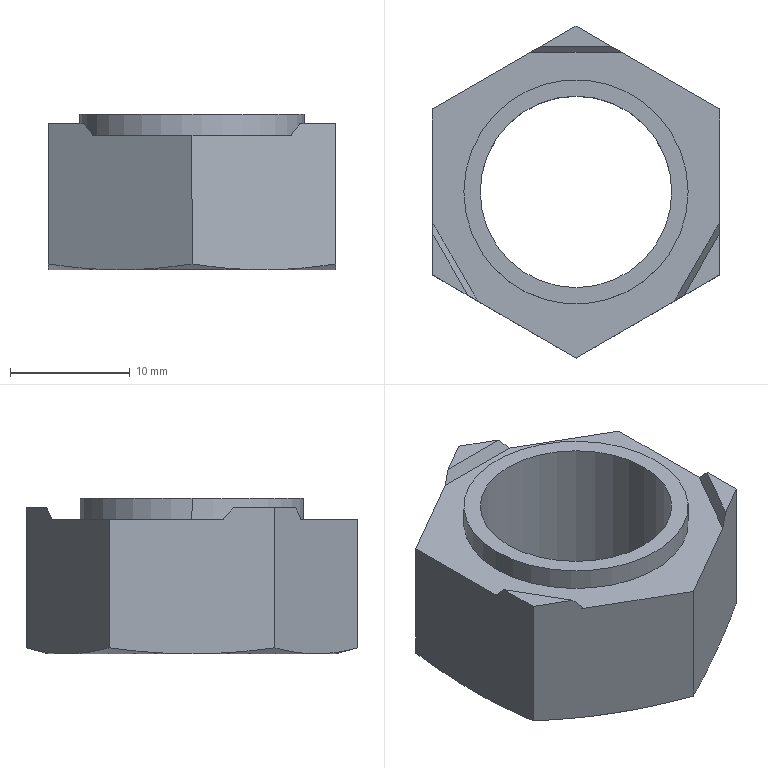Part | SolidWorks | features Cut 3, Boss 1, CirPattern 1, Extrusion 1, RefAxis 1 | 1 solid | 28 faces | box 24 x 27.713 x 13 mm | volume 3465 mm3 | plane 16 | cylinder 6 | cone 6 | commonest cylinder face diameters 16 x2 18.735 x2 19.13 x2
STEP:
#1=CARTESIAN_POINT('',(9.565,0.,0.2));
#2=VERTEX_POINT('',#1);
#3=CARTESIAN_POINT('',(-9.565,0.,0.2));
#4=VERTEX_POINT('',#3);
#5=CARTESIAN_POINT('',(0.,0.,0.2));
#6=DIRECTION('',(0.,0.,-1.));
#7=DIRECTION('',(-1.,0.,0.));
#8=AXIS2_PLACEMENT_3D('',#5,#6,#7);
#9=CIRCLE('',#8,9.565);
#10=EDGE_CURVE('',#2,#4,#9,.T.);
#11=ORIENTED_EDGE('',*,*,#10,.F.);
#12=CARTESIAN_POINT('',(9.565,0.,0.));
#13=VERTEX_POINT('',#12);
#14=CARTESIAN_POINT('',(9.565,0.,0.2));
#15=DIRECTION('',(0.,0.,-1.));
#16=VECTOR('',#15,1000.);
#17=LINE('',#14,#16);
#18=EDGE_CURVE('',#2,#13,#17,.T.);
#19=ORIENTED_EDGE('',*,*,#18,.T.);
#20=CARTESIAN_POINT('',(-9.565,0.,0.));
#21=VERTEX_POINT('',#20);
#22=CARTESIAN_POINT('',(0.,0.,0.));
#23=DIRECTION('',(0.,0.,-1.));
#24=DIRECTION('',(-1.,0.,0.));
#25=AXIS2_PLACEMENT_3D('',#22,#23,#24);
#26=CIRCLE('',#25,9.565);
#27=EDGE_CURVE('',#13,#21,#26,.T.);
#28=ORIENTED_EDGE('',*,*,#27,.T.);
#29=CARTESIAN_POINT('',(-9.565,0.,0.2));
#30=DIRECTION('',(0.,0.,-1.));
#31=VECTOR('',#30,1000.);
#32=LINE('',#29,#31);
#33=EDGE_CURVE('',#4,#21,#32,.T.);
#34=ORIENTED_EDGE('',*,*,#33,.F.);
#35=EDGE_LOOP('',(#11,#19,#28,#34));
#36=FACE_OUTER_BOUND('',#35,.T.);
#37=CARTESIAN_POINT('',(0.,0.,0.2));
#38=DIRECTION('',(0.,0.,-1.));
#39=DIRECTION('',(-1.,0.,0.));
#40=AXIS2_PLACEMENT_3D('',#37,#38,#39);
#41=CYLINDRICAL_SURFACE('',#40,9.565);
#42=ADVANCED_FACE('',(#36),#41,.F.);
#43=CARTESIAN_POINT('',(9.368,0.,13.));
#44=VERTEX_POINT('',#43);
#45=CARTESIAN_POINT('',(-9.367,0.,13.));
#46=VERTEX_POINT('',#45);
#47=CARTESIAN_POINT('',(0.,0.,13.));
#48=DIRECTION('',(0.,0.,1.));
#49=DIRECTION('',(1.,0.,0.));
#50=AXIS2_PLACEMENT_3D('',#47,#48,#49);
#51=CIRCLE('',#50,9.367);
#52=EDGE_CURVE('',#44,#46,#51,.T.);
#53=ORIENTED_EDGE('',*,*,#52,.F.);
#54=CARTESIAN_POINT('',(9.368,0.,11.2));
#55=VERTEX_POINT('',#54);
#56=CARTESIAN_POINT('',(9.367,0.,13.));
#57=DIRECTION('',(0.,0.,-1.));
#58=VECTOR('',#57,1000.);
#59=LINE('',#56,#58);
#60=EDGE_CURVE('',#44,#55,#59,.T.);
#61=ORIENTED_EDGE('',*,*,#60,.T.);
#62=CARTESIAN_POINT('',(-9.367,0.,11.2));
#63=VERTEX_POINT('',#62);
#64=CARTESIAN_POINT('',(0.,0.,11.2));
#65=DIRECTION('',(0.,0.,1.));
#66=DIRECTION('',(-1.,0.,0.));
#67=AXIS2_PLACEMENT_3D('',#64,#65,#66);
#68=CIRCLE('',#67,9.367);
#69=EDGE_CURVE('',#55,#63,#68,.T.);
#70=ORIENTED_EDGE('',*,*,#69,.T.);
#71=CARTESIAN_POINT('',(-9.367,0.,13.));
#72=DIRECTION('',(0.,0.,-1.));
#73=VECTOR('',#72,1000.);
#74=LINE('',#71,#73);
#75=EDGE_CURVE('',#46,#63,#74,.T.);
#76=ORIENTED_EDGE('',*,*,#75,.F.);
#77=EDGE_LOOP('',(#53,#61,#70,#76));
#78=FACE_OUTER_BOUND('',#77,.T.);
#79=CARTESIAN_POINT('',(0.,0.,13.));
#80=DIRECTION('',(0.,0.,-1.));
#81=DIRECTION('',(-1.,0.,0.));
#82=AXIS2_PLACEMENT_3D('',#79,#80,#81);
#83=CYLINDRICAL_SURFACE('',#82,9.367);
#84=ADVANCED_FACE('',(#78),#83,.T.);
#85=CARTESIAN_POINT('',(-8.,0.,13.));
#86=VERTEX_POINT('',#85);
#87=CARTESIAN_POINT('',(8.,0.,13.));
#88=VERTEX_POINT('',#87);
#89=CARTESIAN_POINT('',(0.,0.,13.));
#90=DIRECTION('',(0.,0.,1.));
#91=DIRECTION('',(1.,0.,0.));
#92=AXIS2_PLACEMENT_3D('',#89,#90,#91);
#93=CIRCLE('',#92,8.);
#94=EDGE_CURVE('',#86,#88,#93,.T.);
#95=ORIENTED_EDGE('',*,*,#94,.T.);
#96=CARTESIAN_POINT('',(8.,0.,0.2));
#97=VERTEX_POINT('',#96);
#98=CARTESIAN_POINT('',(8.,0.,13.));
#99=DIRECTION('',(0.,0.,-1.));
#100=VECTOR('',#99,1000.);
#101=LINE('',#98,#100);
#102=EDGE_CURVE('',#88,#97,#101,.T.);
#103=ORIENTED_EDGE('',*,*,#102,.T.);
#104=CARTESIAN_POINT('',(-8.,0.,0.2));
#105=VERTEX_POINT('',#104);
#106=CARTESIAN_POINT('',(0.,0.,0.2));
#107=DIRECTION('',(0.,0.,-1.));
#108=DIRECTION('',(-1.,0.,0.));
#109=AXIS2_PLACEMENT_3D('',#106,#107,#108);
#110=CIRCLE('',#109,8.);
#111=EDGE_CURVE('',#97,#105,#110,.T.);
#112=ORIENTED_EDGE('',*,*,#111,.T.);
#113=CARTESIAN_POINT('',(-8.,0.,13.));
#114=DIRECTION('',(0.,0.,-1.));
#115=VECTOR('',#114,1000.);
#116=LINE('',#113,#115);
#117=EDGE_CURVE('',#86,#105,#116,.T.);
#118=ORIENTED_EDGE('',*,*,#117,.F.);
#119=EDGE_LOOP('',(#95,#103,#112,#118));
#120=FACE_OUTER_BOUND('',#119,.T.);
#121=CARTESIAN_POINT('',(0.,0.,13.));
#122=DIRECTION('',(0.,0.,-1.));
#123=DIRECTION('',(-1.,0.,0.));
#124=AXIS2_PLACEMENT_3D('',#121,#122,#123);
#125=CYLINDRICAL_SURFACE('',#124,8.);
#126=ADVANCED_FACE('',(#120),#125,.F.);
#127=ORIENTED_EDGE('',*,*,#102,.F.);
#128=CARTESIAN_POINT('',(0.,0.,13.));
#129=DIRECTION('',(0.,0.,1.));
#130=DIRECTION('',(1.,0.,0.));
#131=AXIS2_PLACEMENT_3D('',#128,#129,#130);
#132=CIRCLE('',#131,8.);
#133=EDGE_CURVE('',#88,#86,#132,.T.);
#134=ORIENTED_EDGE('',*,*,#133,.T.);
#135=ORIENTED_EDGE('',*,*,#117,.T.);
#136=CARTESIAN_POINT('',(0.,0.,0.2));
#137=DIRECTION('',(0.,0.,-1.));
#138=DIRECTION('',(-1.,0.,0.));
#139=AXIS2_PLACEMENT_3D('',#136,#137,#138);
#140=CIRCLE('',#139,8.);
#141=EDGE_CURVE('',#105,#97,#140,.T.);
#142=ORIENTED_EDGE('',*,*,#141,.T.);
#143=EDGE_LOOP('',(#127,#134,#135,#142));
#144=FACE_OUTER_BOUND('',#143,.T.);
#145=CARTESIAN_POINT('',(0.,0.,13.));
#146=DIRECTION('',(0.,0.,-1.));
#147=DIRECTION('',(-1.,0.,0.));
#148=AXIS2_PLACEMENT_3D('',#145,#146,#147);
#149=CYLINDRICAL_SURFACE('',#148,8.);
#150=ADVANCED_FACE('',(#144),#149,.F.);
#151=CARTESIAN_POINT('',(0.,0.,0.));
#152=DIRECTION('',(0.,0.,-1.));
#153=DIRECTION('',(-1.,0.,0.));
#154=AXIS2_PLACEMENT_3D('',#151,#152,#153);
#155=CIRCLE('',#154,9.565);
#156=EDGE_CURVE('',#21,#13,#155,.T.);
#157=ORIENTED_EDGE('',*,*,#156,.F.);
#158=ORIENTED_EDGE('',*,*,#27,.F.);
#159=EDGE_LOOP('',(#157,#158));
#160=FACE_BOUND('',#159,.T.);
#161=CARTESIAN_POINT('',(-6.,-10.392,0.));
#162=VERTEX_POINT('',#161);
#163=CARTESIAN_POINT('',(-12.,0.,0.));
#164=VERTEX_POINT('',#163);
#165=CARTESIAN_POINT('',(0.,0.,0.));
#166=DIRECTION('',(0.,0.,-1.));
#167=DIRECTION('',(-1.,0.,0.));
#168=AXIS2_PLACEMENT_3D('',#165,#166,#167);
#169=CIRCLE('',#168,12.);
#170=EDGE_CURVE('',#162,#164,#169,.T.);
#171=ORIENTED_EDGE('',*,*,#170,.T.);
#172=CARTESIAN_POINT('',(-6.,10.392,0.));
#173=VERTEX_POINT('',#172);
#174=CARTESIAN_POINT('',(0.,0.,0.));
#175=DIRECTION('',(0.,0.,-1.));
#176=DIRECTION('',(-1.,0.,0.));
#177=AXIS2_PLACEMENT_3D('',#174,#175,#176);
#178=CIRCLE('',#177,12.);
#179=EDGE_CURVE('',#164,#173,#178,.T.);
#180=ORIENTED_EDGE('',*,*,#179,.T.);
#181=CARTESIAN_POINT('',(6.,10.392,0.));
#182=VERTEX_POINT('',#181);
#183=CARTESIAN_POINT('',(0.,0.,0.));
#184=DIRECTION('',(0.,0.,-1.));
#185=DIRECTION('',(-1.,0.,0.));
#186=AXIS2_PLACEMENT_3D('',#183,#184,#185);
#187=CIRCLE('',#186,12.);
#188=EDGE_CURVE('',#173,#182,#187,.T.);
#189=ORIENTED_EDGE('',*,*,#188,.T.);
#190=CARTESIAN_POINT('',(12.,0.,0.));
#191=VERTEX_POINT('',#190);
#192=CARTESIAN_POINT('',(0.,0.,0.));
#193=DIRECTION('',(0.,0.,-1.));
#194=DIRECTION('',(-1.,0.,0.));
#195=AXIS2_PLACEMENT_3D('',#192,#193,#194);
#196=CIRCLE('',#195,12.);
#197=EDGE_CURVE('',#182,#191,#196,.T.);
#198=ORIENTED_EDGE('',*,*,#197,.T.);
#199=CARTESIAN_POINT('',(6.,-10.392,0.));
#200=VERTEX_POINT('',#199);
#201=CARTESIAN_POINT('',(0.,0.,0.));
#202=DIRECTION('',(0.,0.,-1.));
#203=DIRECTION('',(-1.,0.,0.));
#204=AXIS2_PLACEMENT_3D('',#201,#202,#203);
#205=CIRCLE('',#204,12.);
#206=EDGE_CURVE('',#191,#200,#205,.T.);
#207=ORIENTED_EDGE('',*,*,#206,.T.);
#208=CARTESIAN_POINT('',(0.,0.,0.));
#209=DIRECTION('',(0.,0.,-1.));
#210=DIRECTION('',(-1.,0.,0.));
#211=AXIS2_PLACEMENT_3D('',#208,#209,#210);
#212=CIRCLE('',#211,12.);
#213=EDGE_CURVE('',#200,#162,#212,.T.);
#214=ORIENTED_EDGE('',*,*,#213,.T.);
#215=EDGE_LOOP('',(#171,#180,#189,#198,#207,#214));
#216=FACE_OUTER_BOUND('',#215,.T.);
#217=CARTESIAN_POINT('',(12.,6.928,0.));
#218=DIRECTION('',(0.,0.,-1.));
#219=DIRECTION('',(-1.,0.,0.));
#220=AXIS2_PLACEMENT_3D('',#217,#218,#219);
#221=PLANE('',#220);
#222=ADVANCED_FACE('',(#160,#216),#221,.T.);
#223=CARTESIAN_POINT('',(0.,13.856,0.4974));
#224=VERTEX_POINT('',#223);
#225=CARTESIAN_POINT('',(0.,13.856,0.4974));
#226=CARTESIAN_POINT('',(1.,13.279,0.3427));
#227=CARTESIAN_POINT('',(2.,12.702,0.2171));
#228=CARTESIAN_POINT('',(4.,11.547,0.04548));
#229=CARTESIAN_POINT('',(5.,10.97,0.));
#230=CARTESIAN_POINT('',(6.,10.392,0.));
#231=B_SPLINE_CURVE_WITH_KNOTS('',3,(#225,#226,#227,#228,#229,#230),.UNSPECIFIED.,.F.,.F.,(4,2,4),(0.000000231,0.003464,0.006928),.UNSPECIFIED.);
#232=EDGE_CURVE('',#224,#182,#231,.T.);
#233=ORIENTED_EDGE('',*,*,#232,.F.);
#234=CARTESIAN_POINT('',(0.,13.856,12.2));
#235=VERTEX_POINT('',#234);
#236=CARTESIAN_POINT('',(0.,13.856,13.));
#237=DIRECTION('',(0.,0.,-1.));
#238=VECTOR('',#237,1000.);
#239=LINE('',#236,#238);
#240=EDGE_CURVE('',#235,#224,#239,.T.);
#241=ORIENTED_EDGE('',*,*,#240,.F.);
#242=CARTESIAN_POINT('',(2.985,12.133,12.2));
#243=VERTEX_POINT('',#242);
#244=CARTESIAN_POINT('',(12.,6.928,12.2));
#245=DIRECTION('',(0.866,-0.5,0.));
#246=VECTOR('',#245,1000.);
#247=LINE('',#244,#246);
#248=EDGE_CURVE('',#235,#243,#247,.T.);
#249=ORIENTED_EDGE('',*,*,#248,.T.);
#250=CARTESIAN_POINT('',(3.793,11.667,11.2));
#251=VERTEX_POINT('',#250);
#252=CARTESIAN_POINT('',(6.833,9.911,7.436));
#253=DIRECTION('',(0.5907,-0.341,-0.7313));
#254=VECTOR('',#253,1000.);
#255=LINE('',#252,#254);
#256=EDGE_CURVE('',#243,#251,#255,.T.);
#257=ORIENTED_EDGE('',*,*,#256,.T.);
#258=CARTESIAN_POINT('',(12.,6.928,11.2));
#259=VERTEX_POINT('',#258);
#260=CARTESIAN_POINT('',(12.,6.928,11.2));
#261=DIRECTION('',(0.866,-0.5,0.));
#262=VECTOR('',#261,1000.);
#263=LINE('',#260,#262);
#264=EDGE_CURVE('',#251,#259,#263,.T.);
#265=ORIENTED_EDGE('',*,*,#264,.T.);
#266=CARTESIAN_POINT('',(12.,6.928,0.4974));
#267=VERTEX_POINT('',#266);
#268=CARTESIAN_POINT('',(12.,6.928,13.));
#269=DIRECTION('',(0.,0.,-1.));
#270=VECTOR('',#269,1000.);
#271=LINE('',#268,#270);
#272=EDGE_CURVE('',#259,#267,#271,.T.);
#273=ORIENTED_EDGE('',*,*,#272,.T.);
#274=CARTESIAN_POINT('',(6.,10.392,0.));
#275=CARTESIAN_POINT('',(7.,9.815,0.));
#276=CARTESIAN_POINT('',(8.,9.238,0.04548));
#277=CARTESIAN_POINT('',(10.,8.083,0.2171));
#278=CARTESIAN_POINT('',(11.,7.506,0.3427));
#279=CARTESIAN_POINT('',(12.,6.928,0.4974));
#280=B_SPLINE_CURVE_WITH_KNOTS('',3,(#274,#275,#276,#277,#278,#279),.UNSPECIFIED.,.F.,.F.,(4,2,4),(0.006928,0.01039,0.01386),.UNSPECIFIED.);
#281=EDGE_CURVE('',#182,#267,#280,.T.);
#282=ORIENTED_EDGE('',*,*,#281,.F.);
#283=EDGE_LOOP('',(#233,#241,#249,#257,#265,#273,#282));
#284=FACE_OUTER_BOUND('',#283,.T.);
#285=CARTESIAN_POINT('',(12.,6.928,13.));
#286=DIRECTION('',(-0.5,-0.866,0.));
#287=DIRECTION('',(0.866,-0.5,0.));
#288=AXIS2_PLACEMENT_3D('',#285,#286,#287);
#289=PLANE('',#288);
#290=ADVANCED_FACE('',(#284),#289,.F.);
#291=CARTESIAN_POINT('',(-12.,6.928,0.4974));
#292=VERTEX_POINT('',#291);
#293=CARTESIAN_POINT('',(-12.,6.928,0.4974));
#294=CARTESIAN_POINT('',(-11.,7.506,0.3427));
#295=CARTESIAN_POINT('',(-10.,8.083,0.2171));
#296=CARTESIAN_POINT('',(-8.,9.238,0.04548));
#297=CARTESIAN_POINT('',(-7.,9.815,0.));
#298=CARTESIAN_POINT('',(-6.,10.392,0.));
#299=B_SPLINE_CURVE_WITH_KNOTS('',3,(#293,#294,#295,#296,#297,#298),.UNSPECIFIED.,.F.,.F.,(4,2,4),(0.000000231,0.003464,0.006928),.UNSPECIFIED.);
#300=EDGE_CURVE('',#292,#173,#299,.T.);
#301=ORIENTED_EDGE('',*,*,#300,.F.);
#302=CARTESIAN_POINT('',(-12.,6.928,11.2));
#303=VERTEX_POINT('',#302);
#304=CARTESIAN_POINT('',(-12.,6.928,13.));
#305=DIRECTION('',(0.,0.,-1.));
#306=VECTOR('',#305,1000.);
#307=LINE('',#304,#306);
#308=EDGE_CURVE('',#303,#292,#307,.T.);
#309=ORIENTED_EDGE('',*,*,#308,.F.);
#310=CARTESIAN_POINT('',(-3.793,11.667,11.2));
#311=VERTEX_POINT('',#310);
#312=CARTESIAN_POINT('',(0.,13.856,11.2));
#313=DIRECTION('',(0.866,0.5,0.));
#314=VECTOR('',#313,1000.);
#315=LINE('',#312,#314);
#316=EDGE_CURVE('',#303,#311,#315,.T.);
#317=ORIENTED_EDGE('',*,*,#316,.T.);
#318=CARTESIAN_POINT('',(-2.985,12.133,12.2));
#319=VERTEX_POINT('',#318);
#320=CARTESIAN_POINT('',(-1.251,13.134,14.347));
#321=DIRECTION('',(0.5907,0.341,0.7313));
#322=VECTOR('',#321,1000.);
#323=LINE('',#320,#322);
#324=EDGE_CURVE('',#311,#319,#323,.T.);
#325=ORIENTED_EDGE('',*,*,#324,.T.);
#326=CARTESIAN_POINT('',(0.,13.856,12.2));
#327=DIRECTION('',(0.866,0.5,0.));
#328=VECTOR('',#327,1000.);
#329=LINE('',#326,#328);
#330=EDGE_CURVE('',#319,#235,#329,.T.);
#331=ORIENTED_EDGE('',*,*,#330,.T.);
#332=ORIENTED_EDGE('',*,*,#240,.T.);
#333=CARTESIAN_POINT('',(-6.,10.392,0.));
#334=CARTESIAN_POINT('',(-5.,10.97,0.));
#335=CARTESIAN_POINT('',(-4.,11.547,0.04548));
#336=CARTESIAN_POINT('',(-2.,12.702,0.2171));
#337=CARTESIAN_POINT('',(-1.,13.279,0.3427));
#338=CARTESIAN_POINT('',(0.,13.856,0.4974));
#339=B_SPLINE_CURVE_WITH_KNOTS('',3,(#333,#334,#335,#336,#337,#338),.UNSPECIFIED.,.F.,.F.,(4,2,4),(0.006928,0.01039,0.01386),.UNSPECIFIED.);
#340=EDGE_CURVE('',#173,#224,#339,.T.);
#341=ORIENTED_EDGE('',*,*,#340,.F.);
#342=EDGE_LOOP('',(#301,#309,#317,#325,#331,#332,#341));
#343=FACE_OUTER_BOUND('',#342,.T.);
#344=CARTESIAN_POINT('',(0.,13.856,13.));
#345=DIRECTION('',(0.5,-0.866,0.));
#346=DIRECTION('',(0.866,0.5,0.));
#347=AXIS2_PLACEMENT_3D('',#344,#345,#346);
#348=PLANE('',#347);
#349=ADVANCED_FACE('',(#343),#348,.F.);
#350=CARTESIAN_POINT('',(-12.,-6.928,0.4974));
#351=VERTEX_POINT('',#350);
#352=CARTESIAN_POINT('',(-12.,-6.928,0.4974));
#353=CARTESIAN_POINT('',(-12.,-5.777,0.3432));
#354=CARTESIAN_POINT('',(-12.,-4.619,0.2171));
#355=CARTESIAN_POINT('',(-12.,-2.308,0.04537));
#356=CARTESIAN_POINT('',(-12.,-1.153,0.));
#357=CARTESIAN_POINT('',(-12.,0.,0.));
#358=B_SPLINE_CURVE_WITH_KNOTS('',3,(#352,#353,#354,#355,#356,#357),.UNSPECIFIED.,.F.,.F.,(4,2,4),(0.01178,0.01526,0.01874),.UNSPECIFIED.);
#359=EDGE_CURVE('',#351,#164,#358,.T.);
#360=ORIENTED_EDGE('',*,*,#359,.F.);
#361=CARTESIAN_POINT('',(-12.,-6.928,12.2));
#362=VERTEX_POINT('',#361);
#363=CARTESIAN_POINT('',(-12.,-6.928,13.));
#364=DIRECTION('',(0.,0.,-1.));
#365=VECTOR('',#364,1000.);
#366=LINE('',#363,#365);
#367=EDGE_CURVE('',#362,#351,#366,.T.);
#368=ORIENTED_EDGE('',*,*,#367,.F.);
#369=CARTESIAN_POINT('',(-12.,-3.481,12.2));
#370=VERTEX_POINT('',#369);
#371=CARTESIAN_POINT('',(-12.,6.928,12.2));
#372=DIRECTION('',(0.,1.,0.));
#373=VECTOR('',#372,1000.);
#374=LINE('',#371,#373);
#375=EDGE_CURVE('',#362,#370,#374,.T.);
#376=ORIENTED_EDGE('',*,*,#375,.T.);
#377=CARTESIAN_POINT('',(-12.,-2.549,11.2));
#378=VERTEX_POINT('',#377);
#379=CARTESIAN_POINT('',(-12.,0.9618,7.436));
#380=DIRECTION('',(0.,0.682,-0.7313));
#381=VECTOR('',#380,1000.);
#382=LINE('',#379,#381);
#383=EDGE_CURVE('',#370,#378,#382,.T.);
#384=ORIENTED_EDGE('',*,*,#383,.T.);
#385=CARTESIAN_POINT('',(-12.,0.,11.2));
#386=DIRECTION('',(0.,1.,0.));
#387=VECTOR('',#386,1000.);
#388=LINE('',#385,#387);
#389=EDGE_CURVE('',#378,#303,#388,.T.);
#390=ORIENTED_EDGE('',*,*,#389,.T.);
#391=ORIENTED_EDGE('',*,*,#308,.T.);
#392=CARTESIAN_POINT('',(-12.,0.,0.));
#393=CARTESIAN_POINT('',(-12.,1.157,0.));
#394=CARTESIAN_POINT('',(-12.,2.313,0.04565));
#395=CARTESIAN_POINT('',(-12.,4.622,0.2174));
#396=CARTESIAN_POINT('',(-12.,5.775,0.343));
#397=CARTESIAN_POINT('',(-12.,6.928,0.4974));
#398=B_SPLINE_CURVE_WITH_KNOTS('',3,(#392,#393,#394,#395,#396,#397),.UNSPECIFIED.,.F.,.F.,(4,2,4),(0.01874,0.02224,0.02573),.UNSPECIFIED.);
#399=EDGE_CURVE('',#164,#292,#398,.T.);
#400=ORIENTED_EDGE('',*,*,#399,.F.);
#401=EDGE_LOOP('',(#360,#368,#376,#384,#390,#391,#400));
#402=FACE_OUTER_BOUND('',#401,.T.);
#403=CARTESIAN_POINT('',(-12.,6.928,13.));
#404=DIRECTION('',(1.,0.,0.));
#405=DIRECTION('',(0.,0.,-1.));
#406=AXIS2_PLACEMENT_3D('',#403,#404,#405);
#407=PLANE('',#406);
#408=ADVANCED_FACE('',(#402),#407,.F.);
#409=CARTESIAN_POINT('',(0.,-13.856,0.4974));
#410=VERTEX_POINT('',#409);
#411=CARTESIAN_POINT('',(0.,-13.856,0.4974));
#412=CARTESIAN_POINT('',(-1.,-13.279,0.3427));
#413=CARTESIAN_POINT('',(-2.,-12.702,0.2171));
#414=CARTESIAN_POINT('',(-4.,-11.547,0.04548));
#415=CARTESIAN_POINT('',(-5.,-10.97,0.));
#416=CARTESIAN_POINT('',(-6.,-10.392,0.));
#417=B_SPLINE_CURVE_WITH_KNOTS('',3,(#411,#412,#413,#414,#415,#416),.UNSPECIFIED.,.F.,.F.,(4,2,4),(0.000000231,0.003464,0.006928),.UNSPECIFIED.);
#418=EDGE_CURVE('',#410,#162,#417,.T.);
#419=ORIENTED_EDGE('',*,*,#418,.F.);
#420=CARTESIAN_POINT('',(0.,-13.856,11.2));
#421=VERTEX_POINT('',#420);
#422=CARTESIAN_POINT('',(0.,-13.856,13.));
#423=DIRECTION('',(0.,0.,-1.));
#424=VECTOR('',#423,1000.);
#425=LINE('',#422,#424);
#426=EDGE_CURVE('',#421,#410,#425,.T.);
#427=ORIENTED_EDGE('',*,*,#426,.F.);
#428=CARTESIAN_POINT('',(-8.207,-9.118,11.2));
#429=VERTEX_POINT('',#428);
#430=CARTESIAN_POINT('',(-12.,-6.928,11.2));
#431=DIRECTION('',(-0.866,0.5,0.));
#432=VECTOR('',#431,1000.);
#433=LINE('',#430,#432);
#434=EDGE_CURVE('',#421,#429,#433,.T.);
#435=ORIENTED_EDGE('',*,*,#434,.T.);
#436=CARTESIAN_POINT('',(-9.015,-8.652,12.2));
#437=VERTEX_POINT('',#436);
#438=CARTESIAN_POINT('',(-10.749,-7.65,14.347));
#439=DIRECTION('',(-0.5907,0.341,0.7313));
#440=VECTOR('',#439,1000.);
#441=LINE('',#438,#440);
#442=EDGE_CURVE('',#429,#437,#441,.T.);
#443=ORIENTED_EDGE('',*,*,#442,.T.);
#444=CARTESIAN_POINT('',(-12.,-6.928,12.2));
#445=DIRECTION('',(-0.866,0.5,0.));
#446=VECTOR('',#445,1000.);
#447=LINE('',#444,#446);
#448=EDGE_CURVE('',#437,#362,#447,.T.);
#449=ORIENTED_EDGE('',*,*,#448,.T.);
#450=ORIENTED_EDGE('',*,*,#367,.T.);
#451=CARTESIAN_POINT('',(-6.,-10.392,0.));
#452=CARTESIAN_POINT('',(-7.,-9.815,0.));
#453=CARTESIAN_POINT('',(-8.,-9.238,0.04548));
#454=CARTESIAN_POINT('',(-10.,-8.083,0.2171));
#455=CARTESIAN_POINT('',(-11.,-7.506,0.3427));
#456=CARTESIAN_POINT('',(-12.,-6.928,0.4974));
#457=B_SPLINE_CURVE_WITH_KNOTS('',3,(#451,#452,#453,#454,#455,#456),.UNSPECIFIED.,.F.,.F.,(4,2,4),(0.006928,0.01039,0.01386),.UNSPECIFIED.);
#458=EDGE_CURVE('',#162,#351,#457,.T.);
#459=ORIENTED_EDGE('',*,*,#458,.F.);
#460=EDGE_LOOP('',(#419,#427,#435,#443,#449,#450,#459));
#461=FACE_OUTER_BOUND('',#460,.T.);
#462=CARTESIAN_POINT('',(-12.,-6.928,13.));
#463=DIRECTION('',(0.5,0.866,0.));
#464=DIRECTION('',(-0.866,0.5,0.));
#465=AXIS2_PLACEMENT_3D('',#462,#463,#464);
#466=PLANE('',#465);
#467=ADVANCED_FACE('',(#461),#466,.F.);
#468=CARTESIAN_POINT('',(12.,-6.928,0.4974));
#469=VERTEX_POINT('',#468);
#470=CARTESIAN_POINT('',(12.,-6.928,0.4974));
#471=CARTESIAN_POINT('',(11.,-7.506,0.3427));
#472=CARTESIAN_POINT('',(10.,-8.083,0.2171));
#473=CARTESIAN_POINT('',(8.,-9.238,0.04548));
#474=CARTESIAN_POINT('',(7.,-9.815,0.));
#475=CARTESIAN_POINT('',(6.,-10.392,0.));
#476=B_SPLINE_CURVE_WITH_KNOTS('',3,(#470,#471,#472,#473,#474,#475),.UNSPECIFIED.,.F.,.F.,(4,2,4),(0.000000231,0.003464,0.006928),.UNSPECIFIED.);
#477=EDGE_CURVE('',#469,#200,#476,.T.);
#478=ORIENTED_EDGE('',*,*,#477,.F.);
#479=CARTESIAN_POINT('',(12.,-6.928,12.2));
#480=VERTEX_POINT('',#479);
#481=CARTESIAN_POINT('',(12.,-6.928,13.));
#482=DIRECTION('',(0.,0.,-1.));
#483=VECTOR('',#482,1000.);
#484=LINE('',#481,#483);
#485=EDGE_CURVE('',#480,#469,#484,.T.);
#486=ORIENTED_EDGE('',*,*,#485,.F.);
#487=CARTESIAN_POINT('',(9.015,-8.652,12.2));
#488=VERTEX_POINT('',#487);
#489=CARTESIAN_POINT('',(0.,-13.856,12.2));
#490=DIRECTION('',(-0.866,-0.5,0.));
#491=VECTOR('',#490,1000.);
#492=LINE('',#489,#491);
#493=EDGE_CURVE('',#480,#488,#492,.T.);
#494=ORIENTED_EDGE('',*,*,#493,.T.);
#495=CARTESIAN_POINT('',(8.207,-9.118,11.2));
#496=VERTEX_POINT('',#495);
#497=CARTESIAN_POINT('',(5.167,-10.873,7.436));
#498=DIRECTION('',(-0.5907,-0.341,-0.7313));
#499=VECTOR('',#498,1000.);
#500=LINE('',#497,#499);
#501=EDGE_CURVE('',#488,#496,#500,.T.);
#502=ORIENTED_EDGE('',*,*,#501,.T.);
#503=CARTESIAN_POINT('',(0.,-13.856,11.2));
#504=DIRECTION('',(-0.866,-0.5,0.));
#505=VECTOR('',#504,1000.);
#506=LINE('',#503,#505);
#507=EDGE_CURVE('',#496,#421,#506,.T.);
#508=ORIENTED_EDGE('',*,*,#507,.T.);
#509=ORIENTED_EDGE('',*,*,#426,.T.);
#510=CARTESIAN_POINT('',(6.,-10.392,0.));
#511=CARTESIAN_POINT('',(5.,-10.97,0.));
#512=CARTESIAN_POINT('',(4.,-11.547,0.04548));
#513=CARTESIAN_POINT('',(2.,-12.702,0.2171));
#514=CARTESIAN_POINT('',(1.,-13.279,0.3427));
#515=CARTESIAN_POINT('',(0.,-13.856,0.4974));
#516=B_SPLINE_CURVE_WITH_KNOTS('',3,(#510,#511,#512,#513,#514,#515),.UNSPECIFIED.,.F.,.F.,(4,2,4),(0.006928,0.01039,0.01386),.UNSPECIFIED.);
#517=EDGE_CURVE('',#200,#410,#516,.T.);
#518=ORIENTED_EDGE('',*,*,#517,.F.);
#519=EDGE_LOOP('',(#478,#486,#494,#502,#508,#509,#518));
#520=FACE_OUTER_BOUND('',#519,.T.);
#521=CARTESIAN_POINT('',(0.,-13.856,13.));
#522=DIRECTION('',(-0.5,0.866,0.));
#523=DIRECTION('',(-0.866,-0.5,0.));
#524=AXIS2_PLACEMENT_3D('',#521,#522,#523);
#525=PLANE('',#524);
#526=ADVANCED_FACE('',(#520),#525,.F.);
#527=CARTESIAN_POINT('',(12.,6.928,0.4974));
#528=CARTESIAN_POINT('',(12.,5.775,0.343));
#529=CARTESIAN_POINT('',(12.,4.622,0.2174));
#530=CARTESIAN_POINT('',(12.,2.313,0.04565));
#531=CARTESIAN_POINT('',(12.,1.157,0.));
#532=CARTESIAN_POINT('',(12.,0.,0.));
#533=B_SPLINE_CURVE_WITH_KNOTS('',3,(#527,#528,#529,#530,#531,#532),.UNSPECIFIED.,.F.,.F.,(4,2,4),(0.03545,0.03894,0.04242),.UNSPECIFIED.);
#534=EDGE_CURVE('',#267,#191,#533,.T.);
#535=ORIENTED_EDGE('',*,*,#534,.F.);
#536=ORIENTED_EDGE('',*,*,#272,.F.);
#537=CARTESIAN_POINT('',(12.,-2.549,11.2));
#538=VERTEX_POINT('',#537);
#539=CARTESIAN_POINT('',(12.,0.,11.2));
#540=DIRECTION('',(0.,1.,0.));
#541=VECTOR('',#540,1000.);
#542=LINE('',#539,#541);
#543=EDGE_CURVE('',#538,#259,#542,.T.);
#544=ORIENTED_EDGE('',*,*,#543,.F.);
#545=CARTESIAN_POINT('',(12.,-3.481,12.2));
#546=VERTEX_POINT('',#545);
#547=CARTESIAN_POINT('',(12.,-5.484,14.347));
#548=DIRECTION('',(0.,-0.682,0.7313));
#549=VECTOR('',#548,1000.);
#550=LINE('',#547,#549);
#551=EDGE_CURVE('',#538,#546,#550,.T.);
#552=ORIENTED_EDGE('',*,*,#551,.T.);
#553=CARTESIAN_POINT('',(12.,-6.928,12.2));
#554=DIRECTION('',(0.,-1.,0.));
#555=VECTOR('',#554,1000.);
#556=LINE('',#553,#555);
#557=EDGE_CURVE('',#546,#480,#556,.T.);
#558=ORIENTED_EDGE('',*,*,#557,.T.);
#559=ORIENTED_EDGE('',*,*,#485,.T.);
#560=CARTESIAN_POINT('',(12.,0.,0.));
#561=CARTESIAN_POINT('',(12.,-1.153,0.));
#562=CARTESIAN_POINT('',(12.,-2.308,0.04537));
#563=CARTESIAN_POINT('',(12.,-4.619,0.2171));
#564=CARTESIAN_POINT('',(12.,-5.777,0.3432));
#565=CARTESIAN_POINT('',(12.,-6.928,0.4974));
#566=B_SPLINE_CURVE_WITH_KNOTS('',3,(#560,#561,#562,#563,#564,#565),.UNSPECIFIED.,.F.,.F.,(4,2,4),(0.04242,0.0459,0.04937),.UNSPECIFIED.);
#567=EDGE_CURVE('',#191,#469,#566,.T.);
#568=ORIENTED_EDGE('',*,*,#567,.F.);
#569=EDGE_LOOP('',(#535,#536,#544,#552,#558,#559,#568));
#570=FACE_OUTER_BOUND('',#569,.T.);
#571=CARTESIAN_POINT('',(12.,-6.928,13.));
#572=DIRECTION('',(-1.,0.,0.));
#573=DIRECTION('',(0.,-1.,0.));
#574=AXIS2_PLACEMENT_3D('',#571,#572,#573);
#575=PLANE('',#574);
#576=ADVANCED_FACE('',(#570),#575,.F.);
#577=CARTESIAN_POINT('',(-12.,11.667,11.2));
#578=DIRECTION('',(1.,0.,0.));
#579=VECTOR('',#578,1000.);
#580=LINE('',#577,#579);
#581=EDGE_CURVE('',#311,#251,#580,.T.);
#582=ORIENTED_EDGE('',*,*,#581,.F.);
#583=ORIENTED_EDGE('',*,*,#316,.F.);
#584=ORIENTED_EDGE('',*,*,#389,.F.);
#585=CARTESIAN_POINT('',(-1.104,-21.422,11.2));
#586=DIRECTION('',(-0.5,0.866,0.));
#587=VECTOR('',#586,1000.);
#588=LINE('',#585,#587);
#589=EDGE_CURVE('',#429,#378,#588,.T.);
#590=ORIENTED_EDGE('',*,*,#589,.F.);
#591=ORIENTED_EDGE('',*,*,#434,.F.);
#592=ORIENTED_EDGE('',*,*,#507,.F.);
#593=CARTESIAN_POINT('',(19.104,9.755,11.2));
#594=DIRECTION('',(-0.5,-0.866,0.));
#595=VECTOR('',#594,1000.);
#596=LINE('',#593,#595);
#597=EDGE_CURVE('',#538,#496,#596,.T.);
#598=ORIENTED_EDGE('',*,*,#597,.F.);
#599=ORIENTED_EDGE('',*,*,#543,.T.);
#600=ORIENTED_EDGE('',*,*,#264,.F.);
#601=EDGE_LOOP('',(#582,#583,#584,#590,#591,#592,#598,#599,#600));
#602=FACE_OUTER_BOUND('',#601,.T.);
#603=CARTESIAN_POINT('',(0.,0.,11.2));
#604=DIRECTION('',(0.,0.,1.));
#605=DIRECTION('',(-1.,0.,0.));
#606=AXIS2_PLACEMENT_3D('',#603,#604,#605);
#607=CIRCLE('',#606,9.367);
#608=EDGE_CURVE('',#63,#55,#607,.T.);
#609=ORIENTED_EDGE('',*,*,#608,.F.);
#610=ORIENTED_EDGE('',*,*,#69,.F.);
#611=EDGE_LOOP('',(#609,#610));
#612=FACE_BOUND('',#611,.T.);
#613=CARTESIAN_POINT('',(-12.,0.,11.2));
#614=DIRECTION('',(0.,0.,-1.));
#615=DIRECTION('',(-1.,0.,0.));
#616=AXIS2_PLACEMENT_3D('',#613,#614,#615);
#617=PLANE('',#616);
#618=ADVANCED_FACE('',(#602,#612),#617,.F.);
#619=ORIENTED_EDGE('',*,*,#330,.F.);
#620=CARTESIAN_POINT('',(-12.,12.133,12.2));
#621=DIRECTION('',(1.,0.,0.));
#622=VECTOR('',#621,1000.);
#623=LINE('',#620,#622);
#624=EDGE_CURVE('',#319,#243,#623,.T.);
#625=ORIENTED_EDGE('',*,*,#624,.T.);
#626=ORIENTED_EDGE('',*,*,#248,.F.);
#627=EDGE_LOOP('',(#619,#625,#626));
#628=FACE_OUTER_BOUND('',#627,.T.);
#629=CARTESIAN_POINT('',(-12.,12.133,12.2));
#630=DIRECTION('',(0.,0.,-1.));
#631=DIRECTION('',(-1.,0.,0.));
#632=AXIS2_PLACEMENT_3D('',#629,#630,#631);
#633=PLANE('',#632);
#634=ADVANCED_FACE('',(#628),#633,.F.);
#635=ORIENTED_EDGE('',*,*,#624,.F.);
#636=ORIENTED_EDGE('',*,*,#324,.F.);
#637=ORIENTED_EDGE('',*,*,#581,.T.);
#638=ORIENTED_EDGE('',*,*,#256,.F.);
#639=EDGE_LOOP('',(#635,#636,#637,#638));
#640=FACE_OUTER_BOUND('',#639,.T.);
#641=CARTESIAN_POINT('',(-12.,12.133,12.2));
#642=DIRECTION('',(0.,0.9063,-0.4226));
#643=DIRECTION('',(0.,0.4226,0.9063));
#644=AXIS2_PLACEMENT_3D('',#641,#642,#643);
#645=PLANE('',#644);
#646=ADVANCED_FACE('',(#640),#645,.F.);
#647=ORIENTED_EDGE('',*,*,#448,.F.);
#648=CARTESIAN_POINT('',(-1.508,-21.655,12.2));
#649=DIRECTION('',(-0.5,0.866,0.));
#650=VECTOR('',#649,1000.);
#651=LINE('',#648,#650);
#652=EDGE_CURVE('',#437,#370,#651,.T.);
#653=ORIENTED_EDGE('',*,*,#652,.T.);
#654=ORIENTED_EDGE('',*,*,#375,.F.);
#655=EDGE_LOOP('',(#647,#653,#654));
#656=FACE_OUTER_BOUND('',#655,.T.);
#657=CARTESIAN_POINT('',(-1.508,-21.655,12.2));
#658=DIRECTION('',(0.,0.,-1.));
#659=DIRECTION('',(-1.,0.,0.));
#660=AXIS2_PLACEMENT_3D('',#657,#658,#659);
#661=PLANE('',#660);
#662=ADVANCED_FACE('',(#656),#661,.F.);
#663=ORIENTED_EDGE('',*,*,#652,.F.);
#664=ORIENTED_EDGE('',*,*,#442,.F.);
#665=ORIENTED_EDGE('',*,*,#589,.T.);
#666=ORIENTED_EDGE('',*,*,#383,.F.);
#667=EDGE_LOOP('',(#663,#664,#665,#666));
#668=FACE_OUTER_BOUND('',#667,.T.);
#669=CARTESIAN_POINT('',(-1.508,-21.655,12.2));
#670=DIRECTION('',(-0.7849,-0.4532,-0.4226));
#671=DIRECTION('',(0.5,-0.866,0.));
#672=AXIS2_PLACEMENT_3D('',#669,#670,#671);
#673=PLANE('',#672);
#674=ADVANCED_FACE('',(#668),#673,.F.);
#675=ORIENTED_EDGE('',*,*,#557,.F.);
#676=CARTESIAN_POINT('',(19.508,9.522,12.2));
#677=DIRECTION('',(-0.5,-0.866,0.));
#678=VECTOR('',#677,1000.);
#679=LINE('',#676,#678);
#680=EDGE_CURVE('',#546,#488,#679,.T.);
#681=ORIENTED_EDGE('',*,*,#680,.T.);
#682=ORIENTED_EDGE('',*,*,#493,.F.);
#683=EDGE_LOOP('',(#675,#681,#682));
#684=FACE_OUTER_BOUND('',#683,.T.);
#685=CARTESIAN_POINT('',(19.508,9.522,12.2));
#686=DIRECTION('',(0.,0.,-1.));
#687=DIRECTION('',(-1.,0.,0.));
#688=AXIS2_PLACEMENT_3D('',#685,#686,#687);
#689=PLANE('',#688);
#690=ADVANCED_FACE('',(#684),#689,.F.);
#691=ORIENTED_EDGE('',*,*,#680,.F.);
#692=ORIENTED_EDGE('',*,*,#551,.F.);
#693=ORIENTED_EDGE('',*,*,#597,.T.);
#694=ORIENTED_EDGE('',*,*,#501,.F.);
#695=EDGE_LOOP('',(#691,#692,#693,#694));
#696=FACE_OUTER_BOUND('',#695,.T.);
#697=CARTESIAN_POINT('',(19.508,9.522,12.2));
#698=DIRECTION('',(0.7849,-0.4532,-0.4226));
#699=DIRECTION('',(0.5,0.866,0.));
#700=AXIS2_PLACEMENT_3D('',#697,#698,#699);
#701=PLANE('',#700);
#702=ADVANCED_FACE('',(#696),#701,.F.);
#703=CARTESIAN_POINT('',(0.,0.,13.));
#704=DIRECTION('',(0.,0.,1.));
#705=DIRECTION('',(1.,0.,0.));
#706=AXIS2_PLACEMENT_3D('',#703,#704,#705);
#707=CIRCLE('',#706,9.367);
#708=EDGE_CURVE('',#46,#44,#707,.T.);
#709=ORIENTED_EDGE('',*,*,#708,.T.);
#710=ORIENTED_EDGE('',*,*,#52,.T.);
#711=EDGE_LOOP('',(#709,#710));
#712=FACE_OUTER_BOUND('',#711,.T.);
#713=ORIENTED_EDGE('',*,*,#94,.F.);
#714=ORIENTED_EDGE('',*,*,#133,.F.);
#715=EDGE_LOOP('',(#713,#714));
#716=FACE_BOUND('',#715,.T.);
#717=CARTESIAN_POINT('',(0.,0.,13.));
#718=DIRECTION('',(0.,0.,1.));
#719=DIRECTION('',(1.,0.,0.));
#720=AXIS2_PLACEMENT_3D('',#717,#718,#719);
#721=PLANE('',#720);
#722=ADVANCED_FACE('',(#712,#716),#721,.T.);
#723=ORIENTED_EDGE('',*,*,#60,.F.);
#724=ORIENTED_EDGE('',*,*,#708,.F.);
#725=ORIENTED_EDGE('',*,*,#75,.T.);
#726=ORIENTED_EDGE('',*,*,#608,.T.);
#727=EDGE_LOOP('',(#723,#724,#725,#726));
#728=FACE_OUTER_BOUND('',#727,.T.);
#729=CARTESIAN_POINT('',(0.,0.,13.));
#730=DIRECTION('',(0.,0.,-1.));
#731=DIRECTION('',(-1.,0.,0.));
#732=AXIS2_PLACEMENT_3D('',#729,#730,#731);
#733=CYLINDRICAL_SURFACE('',#732,9.367);
#734=ADVANCED_FACE('',(#728),#733,.T.);
#735=ORIENTED_EDGE('',*,*,#477,.T.);
#736=ORIENTED_EDGE('',*,*,#206,.F.);
#737=ORIENTED_EDGE('',*,*,#567,.T.);
#738=EDGE_LOOP('',(#735,#736,#737));
#739=FACE_OUTER_BOUND('',#738,.T.);
#740=CARTESIAN_POINT('',(0.,0.,0.));
#741=DIRECTION('',(0.,0.,1.));
#742=DIRECTION('',(-1.,0.,0.));
#743=AXIS2_PLACEMENT_3D('',#740,#741,#742);
#744=CONICAL_SURFACE('',#743,12.,1.309);
#745=ADVANCED_FACE('',(#739),#744,.T.);
#746=ORIENTED_EDGE('',*,*,#281,.T.);
#747=ORIENTED_EDGE('',*,*,#534,.T.);
#748=ORIENTED_EDGE('',*,*,#197,.F.);
#749=EDGE_LOOP('',(#746,#747,#748));
#750=FACE_OUTER_BOUND('',#749,.T.);
#751=CARTESIAN_POINT('',(0.,0.,0.));
#752=DIRECTION('',(0.,0.,1.));
#753=DIRECTION('',(-1.,0.,0.));
#754=AXIS2_PLACEMENT_3D('',#751,#752,#753);
#755=CONICAL_SURFACE('',#754,12.,1.309);
#756=ADVANCED_FACE('',(#750),#755,.T.);
#757=ORIENTED_EDGE('',*,*,#418,.T.);
#758=ORIENTED_EDGE('',*,*,#213,.F.);
#759=ORIENTED_EDGE('',*,*,#517,.T.);
#760=EDGE_LOOP('',(#757,#758,#759));
#761=FACE_OUTER_BOUND('',#760,.T.);
#762=CARTESIAN_POINT('',(0.,0.,0.));
#763=DIRECTION('',(0.,0.,1.));
#764=DIRECTION('',(-1.,0.,0.));
#765=AXIS2_PLACEMENT_3D('',#762,#763,#764);
#766=CONICAL_SURFACE('',#765,12.,1.309);
#767=ADVANCED_FACE('',(#761),#766,.T.);
#768=ORIENTED_EDGE('',*,*,#359,.T.);
#769=ORIENTED_EDGE('',*,*,#170,.F.);
#770=ORIENTED_EDGE('',*,*,#458,.T.);
#771=EDGE_LOOP('',(#768,#769,#770));
#772=FACE_OUTER_BOUND('',#771,.T.);
#773=CARTESIAN_POINT('',(0.,0.,0.));
#774=DIRECTION('',(0.,0.,1.));
#775=DIRECTION('',(-1.,0.,0.));
#776=AXIS2_PLACEMENT_3D('',#773,#774,#775);
#777=CONICAL_SURFACE('',#776,12.,1.309);
#778=ADVANCED_FACE('',(#772),#777,.T.);
#779=ORIENTED_EDGE('',*,*,#399,.T.);
#780=ORIENTED_EDGE('',*,*,#300,.T.);
#781=ORIENTED_EDGE('',*,*,#179,.F.);
#782=EDGE_LOOP('',(#779,#780,#781));
#783=FACE_OUTER_BOUND('',#782,.T.);
#784=CARTESIAN_POINT('',(0.,0.,0.));
#785=DIRECTION('',(0.,0.,1.));
#786=DIRECTION('',(-1.,0.,0.));
#787=AXIS2_PLACEMENT_3D('',#784,#785,#786);
#788=CONICAL_SURFACE('',#787,12.,1.309);
#789=ADVANCED_FACE('',(#783),#788,.T.);
#790=ORIENTED_EDGE('',*,*,#340,.T.);
#791=ORIENTED_EDGE('',*,*,#232,.T.);
#792=ORIENTED_EDGE('',*,*,#188,.F.);
#793=EDGE_LOOP('',(#790,#791,#792));
#794=FACE_OUTER_BOUND('',#793,.T.);
#795=CARTESIAN_POINT('',(0.,0.,0.));
#796=DIRECTION('',(0.,0.,1.));
#797=DIRECTION('',(-1.,0.,0.));
#798=AXIS2_PLACEMENT_3D('',#795,#796,#797);
#799=CONICAL_SURFACE('',#798,12.,1.309);
#800=ADVANCED_FACE('',(#794),#799,.T.);
#801=ORIENTED_EDGE('',*,*,#18,.F.);
#802=CARTESIAN_POINT('',(0.,0.,0.2));
#803=DIRECTION('',(0.,0.,-1.));
#804=DIRECTION('',(-1.,0.,0.));
#805=AXIS2_PLACEMENT_3D('',#802,#803,#804);
#806=CIRCLE('',#805,9.565);
#807=EDGE_CURVE('',#4,#2,#806,.T.);
#808=ORIENTED_EDGE('',*,*,#807,.F.);
#809=ORIENTED_EDGE('',*,*,#33,.T.);
#810=ORIENTED_EDGE('',*,*,#156,.T.);
#811=EDGE_LOOP('',(#801,#808,#809,#810));
#812=FACE_OUTER_BOUND('',#811,.T.);
#813=CARTESIAN_POINT('',(0.,0.,0.2));
#814=DIRECTION('',(0.,0.,-1.));
#815=DIRECTION('',(-1.,0.,0.));
#816=AXIS2_PLACEMENT_3D('',#813,#814,#815);
#817=CYLINDRICAL_SURFACE('',#816,9.565);
#818=ADVANCED_FACE('',(#812),#817,.F.);
#819=ORIENTED_EDGE('',*,*,#141,.F.);
#820=ORIENTED_EDGE('',*,*,#111,.F.);
#821=EDGE_LOOP('',(#819,#820));
#822=FACE_BOUND('',#821,.T.);
#823=ORIENTED_EDGE('',*,*,#807,.T.);
#824=ORIENTED_EDGE('',*,*,#10,.T.);
#825=EDGE_LOOP('',(#823,#824));
#826=FACE_OUTER_BOUND('',#825,.T.);
#827=CARTESIAN_POINT('',(0.,0.,0.2));
#828=DIRECTION('',(0.,0.,-1.));
#829=DIRECTION('',(-1.,0.,0.));
#830=AXIS2_PLACEMENT_3D('',#827,#828,#829);
#831=PLANE('',#830);
#832=ADVANCED_FACE('',(#822,#826),#831,.T.);
#833=CLOSED_SHELL('',(#42,#84,#126,#150,#222,#290,#349,#408,#467,#526,#576,#618,#634,#646,#662,#674,#690,#702,#722,#734,#745,#756,#767,#778,#789,#800,#818,#832));
#834=MANIFOLD_SOLID_BREP('',#833);
#835=CARTESIAN_POINT('',(0.,0.,0.));
#836=DIRECTION('',(0.,0.,1.));
#837=DIRECTION('',(1.,0.,0.));
#838=AXIS2_PLACEMENT_3D('',#835,#836,#837);
#839=(LENGTH_UNIT()NAMED_UNIT(*)SI_UNIT(.MILLI.,.METRE.));
#840=UNCERTAINTY_MEASURE_WITH_UNIT(LENGTH_MEASURE(0.00001),#839,'','');
#841=(NAMED_UNIT(*)PLANE_ANGLE_UNIT()SI_UNIT($,.RADIAN.));
#842=(NAMED_UNIT(*)SI_UNIT($,.STERADIAN.)SOLID_ANGLE_UNIT());
#843=(GEOMETRIC_REPRESENTATION_CONTEXT(3)GLOBAL_UNCERTAINTY_ASSIGNED_CONTEXT((#840))GLOBAL_UNIT_ASSIGNED_CONTEXT((#839,#841,#842))REPRESENTATION_CONTEXT('',''));
#844=ADVANCED_BREP_SHAPE_REPRESENTATION('',(#834,#838),#843);